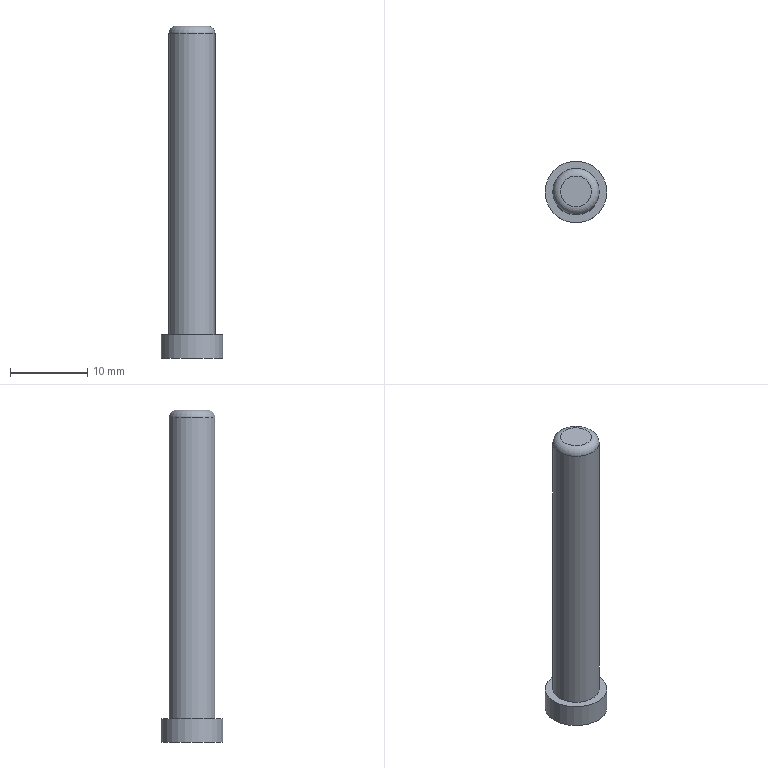Part | NX | features PG_666 2 | 1 solid | 6 faces | box 8 x 8 x 43 mm | volume 1278 mm3 | plane 3 | cylinder 2 | torus 1 | commonest cylinder face diameters 6.001 x1 8 x1
STEP:
#1=CARTESIAN_POINT('',(2822.098,-881.795,862.716));
#2=VERTEX_POINT('',#1);
#3=CARTESIAN_POINT('',(2819.097,-881.795,862.716));
#4=DIRECTION('',(0.,0.,1.));
#5=DIRECTION('',(1.,0.,0.));
#6=AXIS2_PLACEMENT_3D('',#3,#4,#5);
#7=CIRCLE('',#6,3.001);
#8=EDGE_CURVE('',#2,#2,#7,.F.);
#9=ORIENTED_EDGE('',*,*,#8,.T.);
#10=EDGE_LOOP('',(#9));
#11=FACE_BOUND('',#10,.T.);
#12=CARTESIAN_POINT('',(2822.098,-881.795,823.716));
#13=VERTEX_POINT('',#12);
#14=CARTESIAN_POINT('',(2819.097,-881.795,823.716));
#15=DIRECTION('',(0.,0.,1.));
#16=DIRECTION('',(1.,0.,0.));
#17=AXIS2_PLACEMENT_3D('',#14,#15,#16);
#18=CIRCLE('',#17,3.001);
#19=EDGE_CURVE('',#13,#13,#18,.F.);
#20=ORIENTED_EDGE('',*,*,#19,.F.);
#21=EDGE_LOOP('',(#20));
#22=FACE_BOUND('',#21,.T.);
#23=CARTESIAN_POINT('',(2819.097,-881.795,858.716));
#24=DIRECTION('',(0.,0.,-1.));
#25=DIRECTION('',(-1.,0.,0.));
#26=AXIS2_PLACEMENT_3D('',#23,#24,#25);
#27=CYLINDRICAL_SURFACE('',#26,3.001);
#28=ADVANCED_FACE('',(#11,#22),#27,.T.);
#29=CARTESIAN_POINT('',(2821.098,-881.795,863.716));
#30=VERTEX_POINT('',#29);
#31=CARTESIAN_POINT('',(2819.097,-881.795,863.716));
#32=DIRECTION('',(0.,0.,1.));
#33=DIRECTION('',(1.,0.,0.));
#34=AXIS2_PLACEMENT_3D('',#31,#32,#33);
#35=CIRCLE('',#34,2.001);
#36=EDGE_CURVE('',#30,#30,#35,.T.);
#37=ORIENTED_EDGE('',*,*,#36,.T.);
#38=EDGE_LOOP('',(#37));
#39=FACE_BOUND('',#38,.T.);
#40=CARTESIAN_POINT('',(2819.097,-881.795,863.716));
#41=DIRECTION('',(0.,0.,1.));
#42=DIRECTION('',(1.,0.,0.));
#43=AXIS2_PLACEMENT_3D('',#40,#41,#42);
#44=PLANE('',#43);
#45=ADVANCED_FACE('',(#39),#44,.T.);
#46=CARTESIAN_POINT('',(2815.097,-881.795,820.716));
#47=VERTEX_POINT('',#46);
#48=CARTESIAN_POINT('',(2819.097,-881.795,820.716));
#49=DIRECTION('',(0.,0.,1.));
#50=DIRECTION('',(-1.,0.,0.));
#51=AXIS2_PLACEMENT_3D('',#48,#49,#50);
#52=CIRCLE('',#51,4.);
#53=EDGE_CURVE('',#47,#47,#52,.T.);
#54=ORIENTED_EDGE('',*,*,#53,.F.);
#55=EDGE_LOOP('',(#54));
#56=FACE_BOUND('',#55,.T.);
#57=CARTESIAN_POINT('',(2819.097,-881.795,820.716));
#58=DIRECTION('',(0.,0.,-1.));
#59=DIRECTION('',(-1.,0.,0.));
#60=AXIS2_PLACEMENT_3D('',#57,#58,#59);
#61=PLANE('',#60);
#62=ADVANCED_FACE('',(#56),#61,.T.);
#63=ORIENTED_EDGE('',*,*,#19,.T.);
#64=EDGE_LOOP('',(#63));
#65=FACE_BOUND('',#64,.T.);
#66=CARTESIAN_POINT('',(2815.097,-881.795,823.716));
#67=VERTEX_POINT('',#66);
#68=CARTESIAN_POINT('',(2819.097,-881.795,823.716));
#69=DIRECTION('',(0.,0.,-1.));
#70=DIRECTION('',(-1.,0.,0.));
#71=AXIS2_PLACEMENT_3D('',#68,#69,#70);
#72=CIRCLE('',#71,4.);
#73=EDGE_CURVE('',#67,#67,#72,.T.);
#74=ORIENTED_EDGE('',*,*,#73,.F.);
#75=EDGE_LOOP('',(#74));
#76=FACE_BOUND('',#75,.T.);
#77=CARTESIAN_POINT('',(2819.097,-881.795,823.716));
#78=DIRECTION('',(0.,0.,1.));
#79=DIRECTION('',(1.,0.,0.));
#80=AXIS2_PLACEMENT_3D('',#77,#78,#79);
#81=PLANE('',#80);
#82=ADVANCED_FACE('',(#65,#76),#81,.T.);
#83=ORIENTED_EDGE('',*,*,#53,.T.);
#84=EDGE_LOOP('',(#83));
#85=FACE_BOUND('',#84,.T.);
#86=ORIENTED_EDGE('',*,*,#73,.T.);
#87=EDGE_LOOP('',(#86));
#88=FACE_BOUND('',#87,.T.);
#89=CARTESIAN_POINT('',(2819.097,-881.795,823.716));
#90=DIRECTION('',(0.,0.,-1.));
#91=DIRECTION('',(-1.,0.,0.));
#92=AXIS2_PLACEMENT_3D('',#89,#90,#91);
#93=CYLINDRICAL_SURFACE('',#92,4.);
#94=ADVANCED_FACE('',(#85,#88),#93,.T.);
#95=ORIENTED_EDGE('',*,*,#36,.F.);
#96=EDGE_LOOP('',(#95));
#97=FACE_BOUND('',#96,.T.);
#98=ORIENTED_EDGE('',*,*,#8,.F.);
#99=EDGE_LOOP('',(#98));
#100=FACE_BOUND('',#99,.T.);
#101=CARTESIAN_POINT('',(2819.097,-881.795,862.716));
#102=DIRECTION('',(0.,0.,1.));
#103=DIRECTION('',(1.,0.,0.));
#104=AXIS2_PLACEMENT_3D('',#101,#102,#103);
#105=TOROIDAL_SURFACE('',#104,2.001,1.);
#106=ADVANCED_FACE('',(#97,#100),#105,.T.);
#107=CLOSED_SHELL('',(#28,#45,#62,#82,#94,#106));
#108=MANIFOLD_SOLID_BREP('',#107);
#109=(LENGTH_UNIT()NAMED_UNIT(*)SI_UNIT(.MILLI.,.METRE.));
#110=UNCERTAINTY_MEASURE_WITH_UNIT(LENGTH_MEASURE(0.00001),#109,'','');
#111=(NAMED_UNIT(*)PLANE_ANGLE_UNIT()SI_UNIT($,.RADIAN.));
#112=(NAMED_UNIT(*)SI_UNIT($,.STERADIAN.)SOLID_ANGLE_UNIT());
#113=(GEOMETRIC_REPRESENTATION_CONTEXT(3)GLOBAL_UNCERTAINTY_ASSIGNED_CONTEXT((#110))GLOBAL_UNIT_ASSIGNED_CONTEXT((#109,#111,#112))REPRESENTATION_CONTEXT('',''));
#114=ADVANCED_BREP_SHAPE_REPRESENTATION('',(#108),#113);